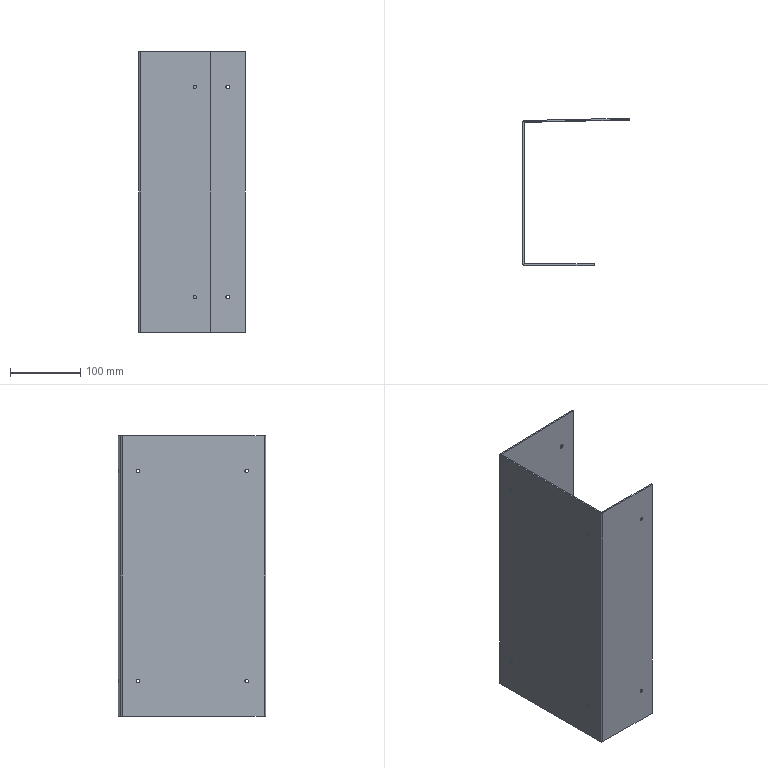Part | STEP file | Assembly TS-S06 | 1 solid | 42 faces | box 151.963 x 210.044 x 400 mm | volume 364106 mm3 | cylinder 24 | plane 18 | commonest cylinder face diameters 5.4 x12 5 x8 0.4 x2 4.4 x2